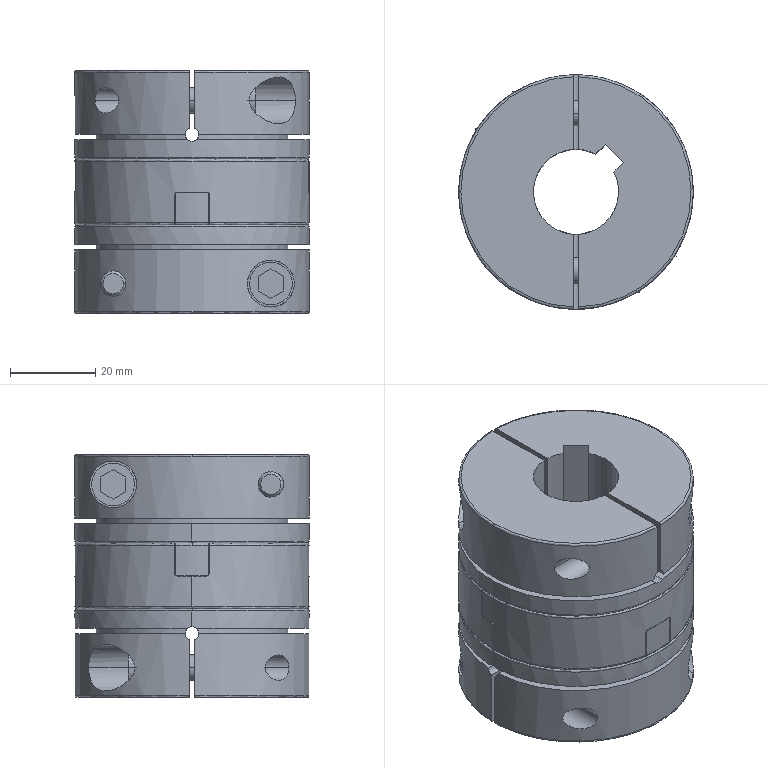Part | SolidWorks | features BaseBody 1 | 1 solid | 228 faces | box 55 x 55 x 57 mm | volume 102625 mm3 | plane 96 | cylinder 94 | spline 19 | cone 19 | commonest cylinder face diameters 1 x16 6 x16 55 x16 7 x8 10 x8 11 x8